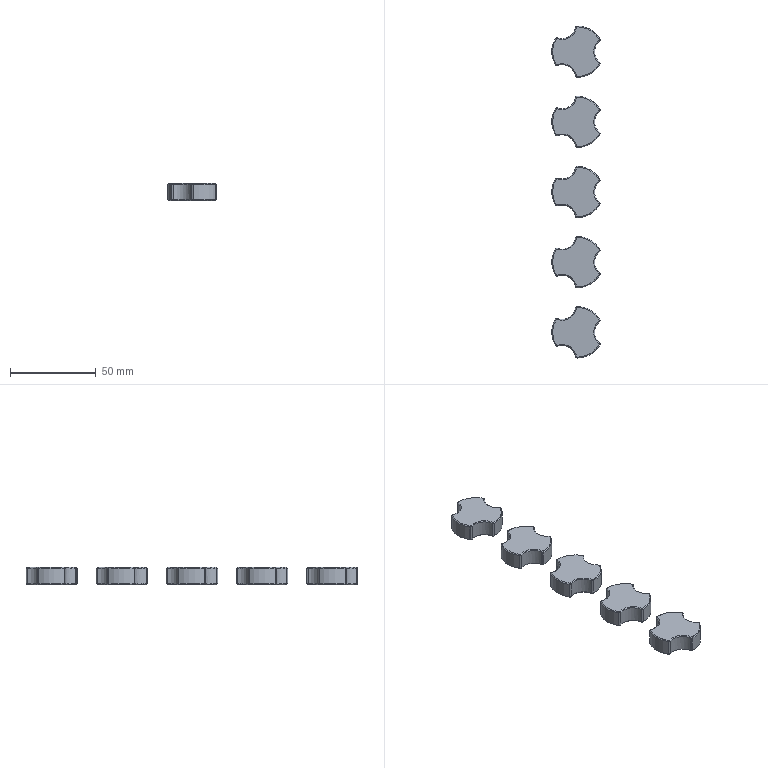NC program | NX | posted with a generic post | part box 28.194 x 194 x 10 mm
Lines 8958 to 9608 of 9608:
(ZLEVEL_PROFILE_COPY_1_COPY , TOOL : D10JING)
N17908 T14 M6
N17910 G54
N17912 G17 G0 G90 X31.494 Y-17.822 S9500 M3
N17914 G43 Z30. H14
N17916 Z-9.
N17918 G94 G1 Z-10. F1000.
N17920 Y-17.28
N17922 G3 X30.994 Y-16.414 R1.
N17924 G1 X30.826 Y-16.316 F1200.
N17926 G2 X28.234 Y-9.115 R6.
N17928 G3 X25.941 Y-5.144 R3.
N17930 G2 X21.001 Y0.701 R6.
N17932 X31.175 Y18.323 R20.
N17934 X38.708 Y16.968 R6.
N17936 G3 X43.292 Y16.968 R3.
N17938 G2 X50.825 Y18.323 R6.
N17940 X60.999 Y0.701 R20.
N17942 X56.059 Y-5.144 R6.
N17944 G3 X53.766 Y-9.115 R3.
N17946 G2 X51.174 Y-16.316 R6.
N17948 X30.994 Y-16.414 R20.
N17950 G3 X29.994 Y-16.414 R1.
N17952 G1 X29.563 Y-16.662
N17954 Z-9.
N17956 G0 Z53.
N17958 X-91.483 Y-17.834
N17960 Z-9.
N17962 G1 Z-10. F1000.
N17964 Y-17.293
N17966 G3 X-91.984 Y-16.427 R1.
N17968 G2 X-92.174 Y-16.316 R20. F1200.
N17970 X-94.766 Y-9.115 R6.
N17972 G3 X-97.059 Y-5.144 R3.
N17974 G2 X-101.999 Y0.701 R6.
N17976 X-91.825 Y18.323 R20.
N17978 X-86.217 Y18.472 R6.
N17980 X-85.877 Y18.293 R5.
N17982 X-84.292 Y16.968 R6.
N17984 G3 X-79.708 Y16.968 R3.
N17986 G2 X-72.175 Y18.323 R6.
N17988 X-62.001 Y0.701 R20.
N17990 X-66.941 Y-5.144 R6.
N17992 G3 X-69.234 Y-9.115 R3.
N17994 G2 X-71.826 Y-16.316 R6.
N17996 X-91.984 Y-16.427 R20.
N17998 G3 X-92.984 Y-16.428 R1.
N18000 G1 X-93.416 Y-16.678
N18002 Z-9.
N18004 G0 Z53.
N18006 X-9.489 Y-17.831
N18008 Z-9.
N18010 G1 Z-10. F1000.
N18012 Y-17.289
N18014 G3 X-9.99 Y-16.424 R1.
N18016 G2 X-10.174 Y-16.316 R20. F1200.
N18018 X-12.766 Y-9.115 R6.
N18020 G3 X-15.059 Y-5.144 R3.
N18022 G2 X-19.999 Y0.701 R6.
N18024 X-9.825 Y18.323 R20.
N18026 X-2.292 Y16.968 R6.
N18028 G3 X2.292 Y16.968 R3.
N18030 G2 X9.825 Y18.323 R6.
N18032 X19.999 Y0.701 R20.
N18034 X15.059 Y-5.144 R6.
N18036 G3 X12.766 Y-9.115 R3.
N18038 G2 X10.174 Y-16.316 R6.
N18040 X-9.99 Y-16.424 R20.
N18042 G3 X-10.99 Y-16.424 R1.
N18044 G1 X-11.422 Y-16.674
N18046 Z-9.
N18048 G0 Z53.
N18050 X72.49 Y-17.821
N18052 Z-9.
N18054 G1 Z-10. F1000.
N18056 X72.491 Y-17.279
N18058 G3 X71.991 Y-16.413 R1.
N18060 G1 X71.826 Y-16.316 F1200.
N18062 G2 X69.234 Y-9.115 R6.
N18064 G3 X66.941 Y-5.144 R3.
N18066 G2 X62.001 Y0.701 R6.
N18068 X72.175 Y18.323 R20.
N18070 X79.708 Y16.968 R6.
N18072 G3 X84.292 Y16.968 R3.
N18074 G2 X91.825 Y18.323 R6.
N18076 X101.999 Y0.701 R20.
N18078 X97.059 Y-5.144 R6.
N18080 G3 X94.766 Y-9.115 R3.
N18082 G2 X92.174 Y-16.316 R6.
N18084 X71.991 Y-16.413 R20.
N18086 G3 X70.991 Y-16.412 R1.
N18088 G1 X70.561 Y-16.66
N18090 Z-9.
N18092 G0 Z53.
N18094 X-50.512 Y-17.82
N18096 Z-9.
N18098 G1 Z-10. F1000.
N18100 X-50.511 Y-17.278
N18102 G3 X-51.011 Y-16.411 R1.
N18104 G1 X-51.174 Y-16.316 F1200.
N18106 G2 X-53.766 Y-9.115 R6.
N18108 G3 X-56.059 Y-5.144 R3.
N18110 G2 X-60.999 Y0.701 R6.
N18112 X-50.825 Y18.323 R20.
N18114 X-43.292 Y16.968 R6.
N18116 G3 X-38.708 Y16.968 R3.
N18118 G2 X-31.175 Y18.323 R6.
N18120 X-21.001 Y0.701 R20.
N18122 X-25.941 Y-5.144 R6.
N18124 G3 X-28.234 Y-9.115 R3.
N18126 G2 X-30.826 Y-16.316 R6.
N18128 X-51.011 Y-16.411 R20.
N18130 G3 X-52.011 Y-16.411 R1.
N18132 G1 X-52.441 Y-16.659
N18134 Z-9.
N18136 G0 Z30.
N18138 M5
(HOLE_MILLING , TOOL : D2)
N18140 T16 M6
N18142 G54
N18144 G17 G0 G90 X82. Y0.903 S9500 M3
N18146 G43 Z30. H16
N18148 Z0.5
N18150 G94 G3 X82.2 Y1.103 R0.2 F1150.
N18152 X82. Y1.303 R0.2
N18154 X82. Y1.303 Z0.35 I0. J-0.4
N18156 X82. Y1.303 Z0.2 I0. J-0.4
N18158 X82. Y1.303 Z0.05 I0. J-0.4
N18160 X82. Y1.303 Z-0.1 I0. J-0.4
N18162 X82. Y1.303 Z-0.25 I0. J-0.4
N18164 X82. Y1.303 Z-0.4 I0. J-0.4
N18166 X82. Y1.303 Z-0.55 I0. J-0.4
N18168 X82. Y1.303 Z-0.7 I0. J-0.4
N18170 X82. Y1.303 Z-0.85 I0. J-0.4
N18172 X82. Y1.303 Z-1. I0. J-0.4
N18174 X82. Y1.303 Z-1.15 I0. J-0.4
N18176 X82. Y1.303 Z-1.3 I0. J-0.4
N18178 X82. Y1.303 Z-1.45 I0. J-0.4
N18180 X82. Y1.303 Z-1.6 I0. J-0.4
N18182 X82. Y1.303 Z-1.75 I0. J-0.4
N18184 X82. Y1.303 Z-1.9 I0. J-0.4
N18186 X82. Y1.303 Z-2.05 I0. J-0.4
N18188 X82. Y1.303 Z-2.2 I0. J-0.4
N18190 X82. Y1.303 Z-2.35 I0. J-0.4
N18192 X82. Y1.303 Z-2.5 I0. J-0.4
N18194 X82. Y1.303 Z-2.65 I0. J-0.4
N18196 X82. Y1.303 Z-2.8 I0. J-0.4
N18198 X82. Y1.303 Z-2.95 I0. J-0.4
N18200 X82. Y1.303 Z-3.1 I0. J-0.4
N18202 X82. Y1.303 Z-3.25 I0. J-0.4
N18204 X82. Y1.303 Z-3.4 I0. J-0.4
N18206 X82. Y1.303 Z-3.55 I0. J-0.4
N18208 X82. Y1.303 Z-3.7 I0. J-0.4
N18210 X82. Y1.303 Z-3.85 I0. J-0.4
N18212 X82. Y1.303 Z-4. I0. J-0.4
N18214 X82. Y1.303 Z-4.15 I0. J-0.4
N18216 X82. Y1.303 Z-4.3 I0. J-0.4
N18218 X82. Y1.303 Z-4.45 I0. J-0.4
N18220 X82. Y1.303 Z-4.6 I0. J-0.4
N18222 X82. Y1.303 Z-4.75 I0. J-0.4
N18224 X82. Y1.303 Z-4.9 I0. J-0.4
N18226 X82. Y1.303 Z-5.05 I0. J-0.4
N18228 X82. Y1.303 Z-5.2 I0. J-0.4
N18230 X82. Y1.303 Z-5.35 I0. J-0.4
N18232 X82. Y1.303 Z-5.5 I0. J-0.4
N18234 X82. Y1.303 Z-5.65 I0. J-0.4
N18236 X82. Y1.303 Z-5.8 I0. J-0.4
N18238 X82. Y1.303 Z-5.95 I0. J-0.4
N18240 X82. Y1.303 Z-6.1 I0. J-0.4
N18242 X82. Y1.303 Z-6.25 I0. J-0.4
N18244 X82. Y1.303 Z-6.4 I0. J-0.4
N18246 X82. Y1.303 Z-6.55 I0. J-0.4
N18248 X82. Y1.303 Z-6.7 I0. J-0.4
N18250 X82. Y1.303 Z-6.85 I0. J-0.4
N18252 X82. Y1.303 Z-7. I0. J-0.4
N18254 X81.6 Y0.903 R0.4
N18256 X82. Y1.303 R-0.4
N18258 X81.8 Y1.103 R0.2
N18260 X82. Y0.903 R0.2
N18262 G0 Z30.
N18264 X41.
N18266 Z0.5
N18268 G3 X41.2 Y1.103 R0.2
N18270 X41. Y1.303 R0.2
N18272 X41. Y1.303 Z0.35 I0. J-0.4
N18274 X41. Y1.303 Z0.2 I0. J-0.4
N18276 X41. Y1.303 Z0.05 I0. J-0.4
N18278 X41. Y1.303 Z-0.1 I0. J-0.4
N18280 X41. Y1.303 Z-0.25 I0. J-0.4
N18282 X41. Y1.303 Z-0.4 I0. J-0.4
N18284 X41. Y1.303 Z-0.55 I0. J-0.4
N18286 X41. Y1.303 Z-0.7 I0. J-0.4
N18288 X41. Y1.303 Z-0.85 I0. J-0.4
N18290 X41. Y1.303 Z-1. I0. J-0.4
N18292 X41. Y1.303 Z-1.15 I0. J-0.4
N18294 X41. Y1.303 Z-1.3 I0. J-0.4
N18296 X41. Y1.303 Z-1.45 I0. J-0.4
N18298 X41. Y1.303 Z-1.6 I0. J-0.4
N18300 X41. Y1.303 Z-1.75 I0. J-0.4
N18302 X41. Y1.303 Z-1.9 I0. J-0.4
N18304 X41. Y1.303 Z-2.05 I0. J-0.4
N18306 X41. Y1.303 Z-2.2 I0. J-0.4
N18308 X41. Y1.303 Z-2.35 I0. J-0.4
N18310 X41. Y1.303 Z-2.5 I0. J-0.4
N18312 X41. Y1.303 Z-2.65 I0. J-0.4
N18314 X41. Y1.303 Z-2.8 I0. J-0.4
N18316 X41. Y1.303 Z-2.95 I0. J-0.4
N18318 X41. Y1.303 Z-3.1 I0. J-0.4
N18320 X41. Y1.303 Z-3.25 I0. J-0.4
N18322 X41. Y1.303 Z-3.4 I0. J-0.4
N18324 X41. Y1.303 Z-3.55 I0. J-0.4
N18326 X41. Y1.303 Z-3.7 I0. J-0.4
N18328 X41. Y1.303 Z-3.85 I0. J-0.4
N18330 X41. Y1.303 Z-4. I0. J-0.4
N18332 X41. Y1.303 Z-4.15 I0. J-0.4
N18334 X41. Y1.303 Z-4.3 I0. J-0.4
N18336 X41. Y1.303 Z-4.45 I0. J-0.4
N18338 X41. Y1.303 Z-4.6 I0. J-0.4
N18340 X41. Y1.303 Z-4.75 I0. J-0.4
N18342 X41. Y1.303 Z-4.9 I0. J-0.4
N18344 X41. Y1.303 Z-5.05 I0. J-0.4
N18346 X41. Y1.303 Z-5.2 I0. J-0.4
N18348 X41. Y1.303 Z-5.35 I0. J-0.4
N18350 X41. Y1.303 Z-5.5 I0. J-0.4
N18352 X41. Y1.303 Z-5.65 I0. J-0.4
N18354 X41. Y1.303 Z-5.8 I0. J-0.4
N18356 X41. Y1.303 Z-5.95 I0. J-0.4
N18358 X41. Y1.303 Z-6.1 I0. J-0.4
N18360 X41. Y1.303 Z-6.25 I0. J-0.4
N18362 X41. Y1.303 Z-6.4 I0. J-0.4
N18364 X41. Y1.303 Z-6.55 I0. J-0.4
N18366 X41. Y1.303 Z-6.7 I0. J-0.4
N18368 X41. Y1.303 Z-6.85 I0. J-0.4
N18370 X41. Y1.303 Z-7. I0. J-0.4
N18372 X40.6 Y0.903 R0.4
N18374 X41. Y1.303 R-0.4
N18376 X40.8 Y1.103 R0.2
N18378 X41. Y0.903 R0.2
N18380 G0 Z30.
N18382 X0.
N18384 Z0.5
N18386 G3 X0.2 Y1.103 R0.2
N18388 X0. Y1.303 R0.2
N18390 X0. Y1.303 Z0.35 I0. J-0.4
N18392 X0. Y1.303 Z0.2 I0. J-0.4
N18394 X0. Y1.303 Z0.05 I0. J-0.4
N18396 X0. Y1.303 Z-0.1 I0. J-0.4
N18398 X0. Y1.303 Z-0.25 I0. J-0.4
N18400 X0. Y1.303 Z-0.4 I0. J-0.4
N18402 X0. Y1.303 Z-0.55 I0. J-0.4
N18404 X0. Y1.303 Z-0.7 I0. J-0.4
N18406 X0. Y1.303 Z-0.85 I0. J-0.4
N18408 X0. Y1.303 Z-1. I0. J-0.4
N18410 X0. Y1.303 Z-1.15 I0. J-0.4
N18412 X0. Y1.303 Z-1.3 I0. J-0.4
N18414 X0. Y1.303 Z-1.45 I0. J-0.4
N18416 X0. Y1.303 Z-1.6 I0. J-0.4
N18418 X0. Y1.303 Z-1.75 I0. J-0.4
N18420 X0. Y1.303 Z-1.9 I0. J-0.4
N18422 X0. Y1.303 Z-2.05 I0. J-0.4
N18424 X0. Y1.303 Z-2.2 I0. J-0.4
N18426 X0. Y1.303 Z-2.35 I0. J-0.4
N18428 X0. Y1.303 Z-2.5 I0. J-0.4
N18430 X0. Y1.303 Z-2.65 I0. J-0.4
N18432 X0. Y1.303 Z-2.8 I0. J-0.4
N18434 X0. Y1.303 Z-2.95 I0. J-0.4
N18436 X0. Y1.303 Z-3.1 I0. J-0.4
N18438 X0. Y1.303 Z-3.25 I0. J-0.4
N18440 X0. Y1.303 Z-3.4 I0. J-0.4
N18442 X0. Y1.303 Z-3.55 I0. J-0.4
N18444 X0. Y1.303 Z-3.7 I0. J-0.4
N18446 X0. Y1.303 Z-3.85 I0. J-0.4
N18448 X0. Y1.303 Z-4. I0. J-0.4
N18450 X0. Y1.303 Z-4.15 I0. J-0.4
N18452 X0. Y1.303 Z-4.3 I0. J-0.4
N18454 X0. Y1.303 Z-4.45 I0. J-0.4
N18456 X0. Y1.303 Z-4.6 I0. J-0.4
N18458 X0. Y1.303 Z-4.75 I0. J-0.4
N18460 X0. Y1.303 Z-4.9 I0. J-0.4
N18462 X0. Y1.303 Z-5.05 I0. J-0.4
N18464 X0. Y1.303 Z-5.2 I0. J-0.4
N18466 X0. Y1.303 Z-5.35 I0. J-0.4
N18468 X0. Y1.303 Z-5.5 I0. J-0.4
N18470 X0. Y1.303 Z-5.65 I0. J-0.4
N18472 X0. Y1.303 Z-5.8 I0. J-0.4
N18474 X0. Y1.303 Z-5.95 I0. J-0.4
N18476 X0. Y1.303 Z-6.1 I0. J-0.4
N18478 X0. Y1.303 Z-6.25 I0. J-0.4
N18480 X0. Y1.303 Z-6.4 I0. J-0.4
N18482 X0. Y1.303 Z-6.55 I0. J-0.4
N18484 X0. Y1.303 Z-6.7 I0. J-0.4
N18486 X0. Y1.303 Z-6.85 I0. J-0.4
N18488 X0. Y1.303 Z-7. I0. J-0.4
N18490 X-0.4 Y0.903 R0.4
N18492 X0. Y1.303 R-0.4
N18494 X-0.2 Y1.103 R0.2
N18496 X0. Y0.903 R0.2
N18498 G0 Z30.
N18500 X-41.
N18502 Z0.5
N18504 G3 X-40.8 Y1.103 R0.2
N18506 X-41. Y1.303 R0.2
N18508 X-41. Y1.303 Z0.35 I0. J-0.4
N18510 X-41. Y1.303 Z0.2 I0. J-0.4
N18512 X-41. Y1.303 Z0.05 I0. J-0.4
N18514 X-41. Y1.303 Z-0.1 I0. J-0.4
N18516 X-41. Y1.303 Z-0.25 I0. J-0.4
N18518 X-41. Y1.303 Z-0.4 I0. J-0.4
N18520 X-41. Y1.303 Z-0.55 I0. J-0.4
N18522 X-41. Y1.303 Z-0.7 I0. J-0.4
N18524 X-41. Y1.303 Z-0.85 I0. J-0.4
N18526 X-41. Y1.303 Z-1. I0. J-0.4
N18528 X-41. Y1.303 Z-1.15 I0. J-0.4
N18530 X-41. Y1.303 Z-1.3 I0. J-0.4
N18532 X-41. Y1.303 Z-1.45 I0. J-0.4
N18534 X-41. Y1.303 Z-1.6 I0. J-0.4
N18536 X-41. Y1.303 Z-1.75 I0. J-0.4
N18538 X-41. Y1.303 Z-1.9 I0. J-0.4
N18540 X-41. Y1.303 Z-2.05 I0. J-0.4
N18542 X-41. Y1.303 Z-2.2 I0. J-0.4
N18544 X-41. Y1.303 Z-2.35 I0. J-0.4
N18546 X-41. Y1.303 Z-2.5 I0. J-0.4
N18548 X-41. Y1.303 Z-2.65 I0. J-0.4
N18550 X-41. Y1.303 Z-2.8 I0. J-0.4
N18552 X-41. Y1.303 Z-2.95 I0. J-0.4
N18554 X-41. Y1.303 Z-3.1 I0. J-0.4
N18556 X-41. Y1.303 Z-3.25 I0. J-0.4
N18558 X-41. Y1.303 Z-3.4 I0. J-0.4
N18560 X-41. Y1.303 Z-3.55 I0. J-0.4
N18562 X-41. Y1.303 Z-3.7 I0. J-0.4
N18564 X-41. Y1.303 Z-3.85 I0. J-0.4
N18566 X-41. Y1.303 Z-4. I0. J-0.4
N18568 X-41. Y1.303 Z-4.15 I0. J-0.4
N18570 X-41. Y1.303 Z-4.3 I0. J-0.4
N18572 X-41. Y1.303 Z-4.45 I0. J-0.4
N18574 X-41. Y1.303 Z-4.6 I0. J-0.4
N18576 X-41. Y1.303 Z-4.75 I0. J-0.4
N18578 X-41. Y1.303 Z-4.9 I0. J-0.4
N18580 X-41. Y1.303 Z-5.05 I0. J-0.4
N18582 X-41. Y1.303 Z-5.2 I0. J-0.4
N18584 X-41. Y1.303 Z-5.35 I0. J-0.4
N18586 X-41. Y1.303 Z-5.5 I0. J-0.4
N18588 X-41. Y1.303 Z-5.65 I0. J-0.4
N18590 X-41. Y1.303 Z-5.8 I0. J-0.4
N18592 X-41. Y1.303 Z-5.95 I0. J-0.4
N18594 X-41. Y1.303 Z-6.1 I0. J-0.4
N18596 X-41. Y1.303 Z-6.25 I0. J-0.4
N18598 X-41. Y1.303 Z-6.4 I0. J-0.4
N18600 X-41. Y1.303 Z-6.55 I0. J-0.4
N18602 X-41. Y1.303 Z-6.7 I0. J-0.4
N18604 X-41. Y1.303 Z-6.85 I0. J-0.4
N18606 X-41. Y1.303 Z-7. I0. J-0.4
N18608 X-41.4 Y0.903 R0.4
N18610 X-41. Y1.303 R-0.4
N18612 X-41.2 Y1.103 R0.2
N18614 X-41. Y0.903 R0.2
N18616 G0 Z30.
N18618 X-82.
N18620 Z0.5
N18622 G3 X-81.8 Y1.103 R0.2
N18624 X-82. Y1.303 R0.2
N18626 X-82. Y1.303 Z0.35 I0. J-0.4
N18628 X-82. Y1.303 Z0.2 I0. J-0.4
N18630 X-82. Y1.303 Z0.05 I0. J-0.4
N18632 X-82. Y1.303 Z-0.1 I0. J-0.4
N18634 X-82. Y1.303 Z-0.25 I0. J-0.4
N18636 X-82. Y1.303 Z-0.4 I0. J-0.4
N18638 X-82. Y1.303 Z-0.55 I0. J-0.4
N18640 X-82. Y1.303 Z-0.7 I0. J-0.4
N18642 X-82. Y1.303 Z-0.85 I0. J-0.4
N18644 X-82. Y1.303 Z-1. I0. J-0.4
N18646 X-82. Y1.303 Z-1.15 I0. J-0.4
N18648 X-82. Y1.303 Z-1.3 I0. J-0.4
N18650 X-82. Y1.303 Z-1.45 I0. J-0.4
N18652 X-82. Y1.303 Z-1.6 I0. J-0.4
N18654 X-82. Y1.303 Z-1.75 I0. J-0.4
N18656 X-82. Y1.303 Z-1.9 I0. J-0.4
N18658 X-82. Y1.303 Z-2.05 I0. J-0.4
N18660 X-82. Y1.303 Z-2.2 I0. J-0.4
N18662 X-82. Y1.303 Z-2.35 I0. J-0.4
N18664 X-82. Y1.303 Z-2.5 I0. J-0.4
N18666 X-82. Y1.303 Z-2.65 I0. J-0.4
N18668 X-82. Y1.303 Z-2.8 I0. J-0.4
N18670 X-82. Y1.303 Z-2.95 I0. J-0.4
N18672 X-82. Y1.303 Z-3.1 I0. J-0.4
N18674 X-82. Y1.303 Z-3.25 I0. J-0.4
N18676 X-82. Y1.303 Z-3.4 I0. J-0.4
N18678 X-82. Y1.303 Z-3.55 I0. J-0.4
N18680 X-82. Y1.303 Z-3.7 I0. J-0.4
N18682 X-82. Y1.303 Z-3.85 I0. J-0.4
N18684 X-82. Y1.303 Z-4. I0. J-0.4
N18686 X-82. Y1.303 Z-4.15 I0. J-0.4
N18688 X-82. Y1.303 Z-4.3 I0. J-0.4
N18690 X-82. Y1.303 Z-4.45 I0. J-0.4
N18692 X-82. Y1.303 Z-4.6 I0. J-0.4
N18694 X-82. Y1.303 Z-4.75 I0. J-0.4
N18696 X-82. Y1.303 Z-4.9 I0. J-0.4
N18698 X-82. Y1.303 Z-5.05 I0. J-0.4
N18700 X-82. Y1.303 Z-5.2 I0. J-0.4
N18702 X-82. Y1.303 Z-5.35 I0. J-0.4
N18704 X-82. Y1.303 Z-5.5 I0. J-0.4
N18706 X-82. Y1.303 Z-5.65 I0. J-0.4
N18708 X-82. Y1.303 Z-5.8 I0. J-0.4
N18710 X-82. Y1.303 Z-5.95 I0. J-0.4
N18712 X-82. Y1.303 Z-6.1 I0. J-0.4
N18714 X-82. Y1.303 Z-6.25 I0. J-0.4
N18716 X-82. Y1.303 Z-6.4 I0. J-0.4
N18718 X-82. Y1.303 Z-6.55 I0. J-0.4
N18720 X-82. Y1.303 Z-6.7 I0. J-0.4
N18722 X-82. Y1.303 Z-6.85 I0. J-0.4
N18724 X-82. Y1.303 Z-7. I0. J-0.4
N18726 X-82.4 Y0.903 R0.4
N18728 X-82. Y1.303 R-0.4
N18730 X-82.2 Y1.103 R0.2
N18732 X-82. Y0.903 R0.2
N18734 G0 Z30.
N18736 M5
(PLANAR_MILL_COPY_COPY_COPY_COPY , TOOL : D6A45)
N18738 T01 M6
N18740 G54
N18742 G17 G0 G90 X82.433 Y1.153 S9500 M3
N18744 G43 Z30. H1
N18746 Z0.
N18748 G94 G1 Z-1.5 F1250.
N18750 G3 X82. Y1.403 R0.5
N18752 X81.5 Y0.903 R0.5
N18754 X82. Y1.403 R-0.5
N18756 X81.567 Y1.153 R0.5
N18758 G1 Z0.
N18760 G0 Z30.
N18762 X89.426 Y15.663
N18764 Z0.
N18766 G1 Z-1.5
N18768 G3 X89.93 Y14.799 R1.
N18770 G1 X90. Y14.759
N18772 G2 X97.999 Y0.741 R16.
N18774 X96.352 Y-1.207 R2.
N18776 G3 X91.004 Y-10.472 R7.
N18778 G2 X90.14 Y-12.872 R2.
N18780 X73.86 Y-12.872 R16.
N18782 X72.996 Y-10.472 R2.
N18784 G3 X67.648 Y-1.207 R7.
N18786 G2 X66.001 Y0.741 R2.
N18788 X74.14 Y14.839 R16.
N18790 X76.651 Y14.387 R2.
N18792 G3 X87.349 Y14.387 R7.
N18794 G2 X89.93 Y14.799 R2.001
N18796 G3 X90.93 Y14.804 R1.
N18798 G1 Z0.
N18800 G0 Z30.
N18802 X41.433 Y1.153
N18804 Z0.
N18806 G1 Z-1.5
N18808 G3 X41. Y1.403 R0.5
N18810 X40.5 Y0.903 R0.5
N18812 X41. Y1.403 R-0.5
N18814 X40.567 Y1.153 R0.5
N18816 G1 Z0.
N18818 G0 Z30.
N18820 X48.426 Y15.663
N18822 Z0.
N18824 G1 Z-1.5
N18826 G3 X48.93 Y14.799 R1.
N18828 G1 X49. Y14.759
N18830 G2 X56.999 Y0.741 R16.
N18832 X55.352 Y-1.207 R2.
N18834 G3 X50.004 Y-10.472 R7.
N18836 G2 X49.14 Y-12.872 R2.
N18838 X32.86 Y-12.872 R16.
N18840 X31.996 Y-10.472 R2.
N18842 G3 X26.648 Y-1.207 R7.
N18844 G2 X25.001 Y0.741 R2.
N18846 X33.14 Y14.839 R16.
N18848 X35.651 Y14.387 R2.
N18850 G3 X46.349 Y14.387 R7.
N18852 G2 X48.93 Y14.799 R2.001
N18854 G3 X49.93 Y14.804 R1.
N18856 G1 Z0.
N18858 G0 Z30.
N18860 X0.433 Y1.153
N18862 Z0.
N18864 G1 Z-1.5
N18866 G3 X0. Y1.403 R0.5
N18868 X-0.5 Y0.903 R0.5
N18870 X0. Y1.403 R-0.5
N18872 X-0.433 Y1.153 R0.5
N18874 G1 Z0.
N18876 G0 Z30.
N18878 X7.426 Y15.663
N18880 Z0.
N18882 G1 Z-1.5
N18884 G3 X7.93 Y14.799 R1.
N18886 G1 X8. Y14.759
N18888 G2 X15.999 Y0.741 R16.
N18890 X14.352 Y-1.207 R2.
N18892 G3 X9.004 Y-10.472 R7.
N18894 G2 X8.14 Y-12.872 R2.
N18896 X-8.14 Y-12.872 R16.
N18898 X-9.004 Y-10.472 R2.
N18900 G3 X-14.352 Y-1.207 R7.
N18902 G2 X-15.999 Y0.741 R2.
N18904 X-7.86 Y14.839 R16.
N18906 X-5.349 Y14.387 R2.
N18908 G3 X5.349 Y14.387 R7.
N18910 G2 X7.93 Y14.799 R2.001
N18912 G3 X8.93 Y14.804 R1.
N18914 G1 Z0.
N18916 G0 Z30.
N18918 X-40.567 Y1.153
N18920 Z0.
N18922 G1 Z-1.5
N18924 G3 X-41. Y1.403 R0.5
N18926 X-41.5 Y0.903 R0.5
N18928 X-41. Y1.403 R-0.5
N18930 X-41.433 Y1.153 R0.5
N18932 G1 Z0.
N18934 G0 Z30.
N18936 X-33.574 Y15.663
N18938 Z0.
N18940 G1 Z-1.5
N18942 G3 X-33.07 Y14.799 R1.
N18944 G1 X-33. Y14.759
N18946 G2 X-25.001 Y0.741 R16.
N18948 X-26.648 Y-1.207 R2.
N18950 G3 X-31.996 Y-10.472 R7.
N18952 G2 X-32.86 Y-12.872 R2.
N18954 X-49.14 Y-12.872 R16.
N18956 X-50.004 Y-10.472 R2.
N18958 G3 X-55.352 Y-1.207 R7.
N18960 G2 X-56.999 Y0.741 R2.
N18962 X-48.86 Y14.839 R16.
N18964 X-46.349 Y14.387 R2.
N18966 G3 X-35.651 Y14.387 R7.
N18968 G2 X-33.07 Y14.799 R2.001
N18970 G3 X-32.07 Y14.804 R1.
N18972 G1 Z0.
N18974 G0 Z30.
N18976 X-81.567 Y1.153
N18978 Z0.
N18980 G1 Z-1.5
N18982 G3 X-82. Y1.403 R0.5
N18984 X-82.5 Y0.903 R0.5
N18986 X-82. Y1.403 R-0.5
N18988 X-82.433 Y1.153 R0.5
N18990 G1 Z0.
N18992 G0 Z30.
N18994 X-74.574 Y15.663
N18996 Z0.
N18998 G1 Z-1.5
N19000 G3 X-74.07 Y14.799 R1.
N19002 G1 X-74. Y14.759
N19004 G2 X-66.001 Y0.741 R16.
N19006 X-67.648 Y-1.207 R2.
N19008 G3 X-72.996 Y-10.472 R7.
N19010 G2 X-73.86 Y-12.872 R2.
N19012 X-90.14 Y-12.872 R16.
N19014 X-91.004 Y-10.472 R2.
N19016 G3 X-96.352 Y-1.207 R7.
N19018 G2 X-97.999 Y0.741 R2.
N19020 X-89.86 Y14.839 R16.
N19022 X-87.349 Y14.387 R2.
N19024 G3 X-76.651 Y14.387 R7.
N19026 G2 X-74.07 Y14.799 R2.001
N19028 G3 X-73.07 Y14.804 R1.
N19030 G1 Z0.
N19032 G0 Z30.
N19034 M5
(刀补17 , TOOL : D2)
N19036 T16 M6
N19038 G54
N19040 G17 G0 G90 X82. Y0.903 S9500 M3
N19042 G43 Z30. H16
N19044 Z0.5
N19046 G41 G94 G1 X82.096 Y0.93 F1150. D16
N19048 G3 X82. Y1.353 R0.222
N19050 X82. Y1.353 Z-1.5 I0. J-0.45
N19052 X82. Y1.353 Z-3.5 I0. J-0.45
N19054 X82. Y1.353 Z-5.5 I0. J-0.45
N19056 X82.45 Y0.903 Z-7. R-0.45
N19058 X82. Y1.353 R0.45
N19060 X82.45 Y0.903 R-0.45
N19062 X82.027 Y0.999 R0.222
N19064 G40
N19066 G1 X82. Y0.903
N19068 G0 Z30.
N19070 X41.
N19072 Z0.5
N19074 G41 G1 X41.096 Y0.93
N19076 G3 X41. Y1.353 R0.222
N19078 X41. Y1.353 Z-1.5 I0. J-0.45
N19080 X41. Y1.353 Z-3.5 I0. J-0.45
N19082 X41. Y1.353 Z-5.5 I0. J-0.45
N19084 X41.45 Y0.903 Z-7. R-0.45
N19086 X41. Y1.353 R0.45
N19088 X41.45 Y0.903 R-0.45
N19090 X41.027 Y0.999 R0.222
N19092 G40
N19094 G1 X41. Y0.903
N19096 G0 Z30.
N19098 X0.
N19100 Z0.5
N19102 G41 G1 X0.096 Y0.93
N19104 G3 X0. Y1.353 R0.222
N19106 X0. Y1.353 Z-1.5 I0. J-0.45
N19108 X0. Y1.353 Z-3.5 I0. J-0.45
N19110 X0. Y1.353 Z-5.5 I0. J-0.45
N19112 X0.45 Y0.903 Z-7. R-0.45
N19114 X0. Y1.353 R0.45
N19116 X0.45 Y0.903 R-0.45
N19118 X0.027 Y0.999 R0.222
N19120 G40
N19122 G1 X0. Y0.903
N19124 G0 Z30.
N19126 X-41.
N19128 Z0.5
N19130 G41 G1 X-40.904 Y0.93
N19132 G3 X-41. Y1.353 R0.222
N19134 X-41. Y1.353 Z-1.5 I0. J-0.45
N19136 X-41. Y1.353 Z-3.5 I0. J-0.45
N19138 X-41. Y1.353 Z-5.5 I0. J-0.45
N19140 X-40.55 Y0.903 Z-7. R-0.45
N19142 X-41. Y1.353 R0.45
N19144 X-40.55 Y0.903 R-0.45
N19146 X-40.973 Y0.999 R0.222
N19148 G40
N19150 G1 X-41. Y0.903
N19152 G0 Z30.
N19154 X-82.
N19156 Z0.5
N19158 G41 G1 X-81.904 Y0.93
N19160 G3 X-82. Y1.353 R0.222
N19162 X-82. Y1.353 Z-1.5 I0. J-0.45
N19164 X-82. Y1.353 Z-3.5 I0. J-0.45
N19166 X-82. Y1.353 Z-5.5 I0. J-0.45
N19168 X-81.55 Y0.903 Z-7. R-0.45
N19170 X-82. Y1.353 R0.45
N19172 X-81.55 Y0.903 R-0.45
N19174 X-81.973 Y0.999 R0.222
N19176 G40
N19178 G1 X-82. Y0.903
N19180 G0 Z30.
N19182 M5
N19184 M2